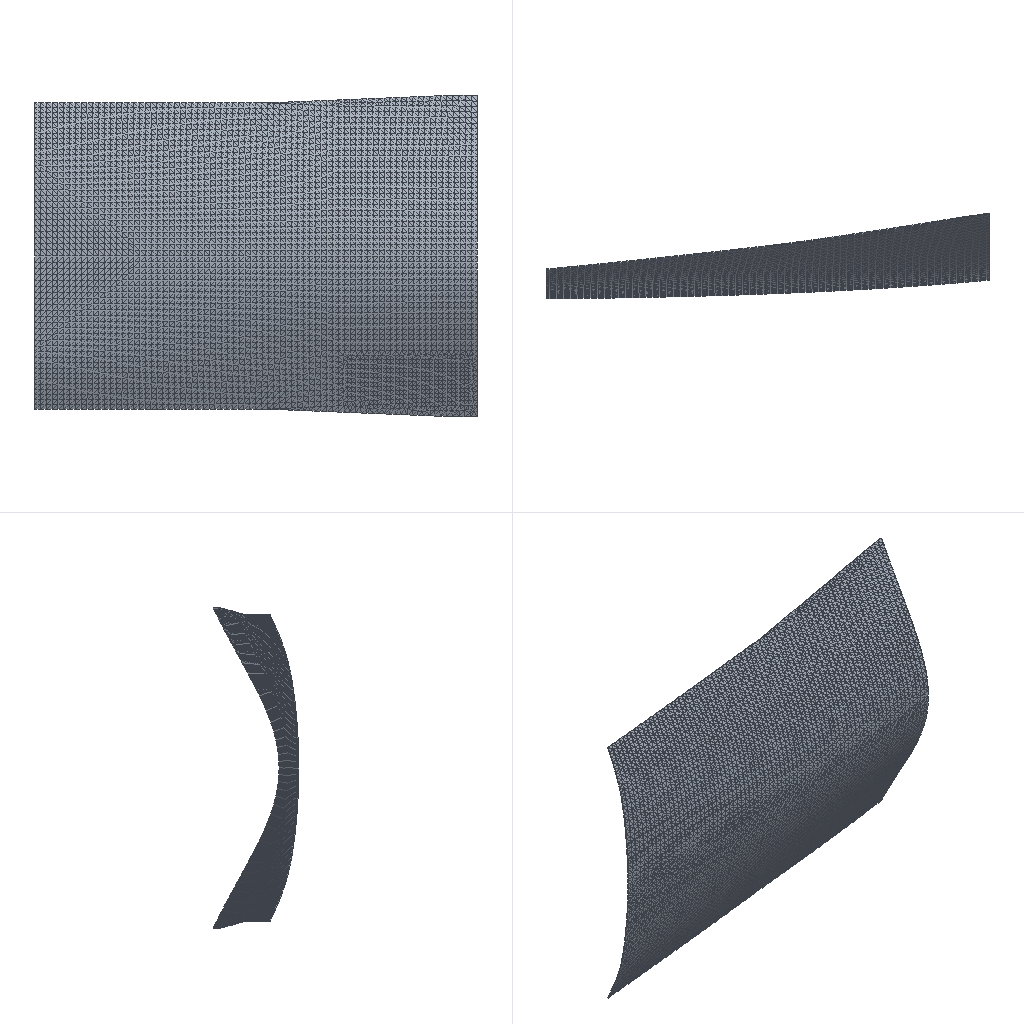Simulation study | abaqus
Set-up summary:
category,name,step,type,value,unit,region
solver,abaqus
solver,version,,,Abaqus/Explicit 2020
units,not stated in the deck,,not stated
analysis,deck,,transient,transient
load_step,Step-1,Step-1,transient
load_step,requested,,,1
mesh,nodes,,,14742
mesh,elements,,,31636
element_type,C3D4,,solid,25997
element_type,R3D3,,rigid,4
element_type,R3D4,,rigid,5635
load,load commands in deck,,count,4
bc,support commands in deck,,count,13
material,MATERIAL-1,,in results
check,setup vs results,,match,"per instance, exact: element labels, types and connectivity; labels of the nodes the elements use; coordinates of those nodes at SINGLE_PRECISION in 2 of 2 instance(s)"
Abaqus input file, long lists of numbers shortened:
*Heading
** Job name: Job-1 Model name: Model-1
** Generated by: Abaqus/CAE 2020
*Preprint, echo=NO, model=NO, history=NO, contact=NO
**
** PARTS
**
*Part, name=FBLJ1-01-1
*Node
      1,   11788.773,   193.464,        -450.
      2,   11859.74,   -368.07,        -450.
** (5822 more lines like these left out)
*Element, type=R3D4
  1,    1,   20,  736,  110
  2,   20,   21,  737,  736
** (5633 more lines like these left out)
*Element, type=R3D3
5513,  466, 5809,  467
5514, 5811, 5800,  686
** (2 more lines like these left out)
*Node
   5825,   12880.093,   331.384, 4.04973298e-06
*Nset, nset=FBLJ1-01-1-RefPt_, internal
5825,
*Elset, elset=FBLJ1-01-1, generate
    1,  5639,     1
*End Part
**
*Part, name=work
*Node
      1,   13047.076,  -171.518,   648.057
      2,   13047.552,  -175.549,         650.
** (8915 more lines like these left out)
*Element, type=C3D4
    1, 8893,  552, 1064,  551
    2,  139,  179,   14, 8894
** (25995 more lines like these left out)
*Nset, nset=Set-5, generate
    1,  8917,     1
*Elset, elset=Set-5, generate
     1,  25997,      1
** Section: Section-1
*Solid Section, elset=Set-5, material=Material-1
,
*End Part
**
**
** ASSEMBLY
**
*Assembly, name=Assembly
**
*Instance, name=FBLJ1-01-1-1, part=FBLJ1-01-1
-12880.093,  -331.384,       -4e-06
*End Instance
**
*Instance, name=work-1, part=work
-12880.093,  -331.384,       -4e-06
*End Instance
**
*Node
      1,   127.547,  -507.531,   648.058
*Node
      2,   127.547,  -507.531,  -648.058
*Nset, nset=Set-2, instance=FBLJ1-01-1-1
 5825,
*Nset, nset=Set-5
 1,
*Nset, nset=Set-6
 2,
*Nset, nset=m_Set-3
 1,
*Nset, nset=m_Set-4
 2,
*Elset, elset=_s_Surf-1_S1, internal, instance=work-1
 13301, 13528, 13800, 14269, 14363, 14473, 14517, 14967, 15049, 15108, 15127, 15355, 15392, 16841, 16958, 17013
 17200, 17387, 17447, 22779
*Elset, elset=_s_Surf-1_S2, internal, instance=work-1
 13394, 14306, 14720, 15064, 15395, 15427, 15473, 16083, 16567, 17079, 17232, 17244, 17258, 17289, 17301, 17337
 17340, 17350, 17405, 22847, 22916
*Elset, elset=_s_Surf-1_S4, internal, instance=work-1
 13472, 14275, 14442, 14506, 14612, 14894, 14895, 14970, 14982, 14990, 15032, 15156, 15163, 15170, 15180, 15315
 15405, 15418, 15428, 15431, 15455, 15460, 15462, 15471, 15474, 15487, 15500, 15508, 16294, 17017, 17218, 17288
** (1 more lines like these left out)
*Elset, elset=_s_Surf-1_S3, internal, instance=work-1
  9855, 12643, 12863, 12878, 13417, 13911, 13992, 14294, 14304, 14385, 14389, 14408, 14409, 14501, 14602, 14613
 14637, 14676, 14699, 14747, 14766, 14791, 14824, 14905, 14934, 14949, 14963, 14965, 14977, 15003, 15007, 15017
** (3 more lines like these left out)
*Surface, type=ELEMENT, name=s_Surf-1
_s_Surf-1_S1, S1
_s_Surf-1_S2, S2
_s_Surf-1_S4, S4
_s_Surf-1_S3, S3
*Elset, elset=_s_Surf-2_S4, internal, instance=work-1
  1238,  1266,  1271,  1405,  1429,  1460,  1871,  3851,  4255,  4265,  4676,  6195,  6646,  6842,  7024,  7043
  7067,  7119,  7156,  7340,  7388,  7456,  7464,  7476,  7477, 14199, 15018, 25456
*Elset, elset=_s_Surf-2_S2, internal, instance=work-1
  1254,  1347,  1351,  1377,  1403,  1423,  1435,  1478,  1517,  1677,  1722,  1726,  1776,  2779,  2790,  4706
  6645,  6936,  7005,  7117,  7270,  7295,  7460,  7473,  8447,  9035,  9042,  9043,  9049, 10150, 12359, 12951
** (1 more lines like these left out)
*Elset, elset=_s_Surf-2_S3, internal, instance=work-1
  1261,  1348,  1364,  1447,  1452,  1702,  2773,  3673,  3713,  4485,  5801,  6356,  6604,  6608,  6713,  6754
  6756,  6802,  6805,  6822,  6911,  6958,  6961,  6963,  7002,  7023,  7202,  7225,  7248,  7287,  7364,  7441
** (1 more lines like these left out)
*Elset, elset=_s_Surf-2_S1, internal, instance=work-1
  1319,  1352,  1366,  1370,  1371,  1395,  1407,  1416,  1419,  1426,  1437,  1441,  1458,  1501,  1731,  3680
  3681,  3976,  6292,  6408,  6666,  6691,  6799,  6910,  7204,  7319,  7471,  7475,  8996,  9009,  9031, 10644
** (1 more lines like these left out)
*Surface, type=ELEMENT, name=s_Surf-2
_s_Surf-2_S4, S4
_s_Surf-2_S2, S2
_s_Surf-2_S3, S3
_s_Surf-2_S1, S1
*Rigid Body, ref node=FBLJ1-01-1-1.FBLJ1-01-1-RefPt_, elset=FBLJ1-01-1-1.FBLJ1-01-1
** Constraint: Constraint-1
*Coupling, constraint name=Constraint-1, ref node=m_Set-3, surface=s_Surf-1
*Kinematic
** Constraint: Constraint-2
*Coupling, constraint name=Constraint-2, ref node=m_Set-4, surface=s_Surf-2
*Kinematic
*End Assembly
*Amplitude, name=Amp-1
             0.,              0.,            0.01,              1.
**
** MATERIALS
**
*Material, name=Material-1
*Density
 2.7e-09,
*Elastic
72000., 0.3
*Plastic
270.,0.
**
** INTERACTION PROPERTIES
**
*Surface Interaction, name=IntProp-1
*Friction
 0.2,
*Surface Behavior, pressure-overclosure=HARD
** ----------------------------------------------------------------
**
** STEP: Step-1
**
*Step, name=Step-1, nlgeom=YES
*Dynamic, Explicit
, 0.01
*Bulk Viscosity
0.06, 1.2
**
** BOUNDARY CONDITIONS
**
** Name: BC-1 Type: 对称/反对称/完全固定
*Boundary
Set-2, ENCASTRE
** Name: [REDACTED] : Displacement/rotation angle
*Boundary, amplitude=Amp-1
Set-5, 1, 1
Set-5, 2, 2, 100.
Set-5, 3, 3, 100.
Set-5, 4, 4
Set-5, 5, 5
Set-5, 6, 6
** Name: [REDACTED] : Displacement/rotation angle
*Boundary, amplitude=Amp-1
Set-6, 1, 1
Set-6, 2, 2, 100.
Set-6, 3, 3, -100.
Set-6, 4, 4
Set-6, 5, 5
Set-6, 6, 6
**
** INTERACTIONS
**
** Interaction: Int-1
*Contact, op=NEW
*Contact Inclusions, ALL EXTERIOR
*Contact Property Assignment
 ,  , IntProp-1
**
** OUTPUT REQUESTS
**
*Restart, write, number interval=1, time marks=NO
**
** FIELD OUTPUT: F-Output-1
**
*Output, field, number interval=50
*Node Output
A, CF, RF, RM, RT, U, UR, UT
V
*Element Output, directions=YES
E, EVF, LE, MISES, MISESMAX, MISESONLY, PE, PEEQ, PEEQMAX, PEEQT, PEEQVAVG, PEMAG, PEQC, PEVAVG, PRESSONLY, S
SF, SSAVG, SVAVG, YIELDPOT
*Contact Output
CDISP, CSTRESS
**
** HISTORY OUTPUT: H-Output-1
**
*Output, history, time interval=1e-07
*Node Output, nset=Set-2
RF1, RF2, RF3
*End Step
Results summary:
result,step,Step-1,completed,increments=148861 time=0.01/0.01
result,analysis,,,transient
result,last_loadstep,,,1
result,primary field,,,U
result,reaction total,,FX,23535.922,model units
result,reaction total,,FY,-113735.0,model units
result,reaction total,,FZ,19711.438,model units